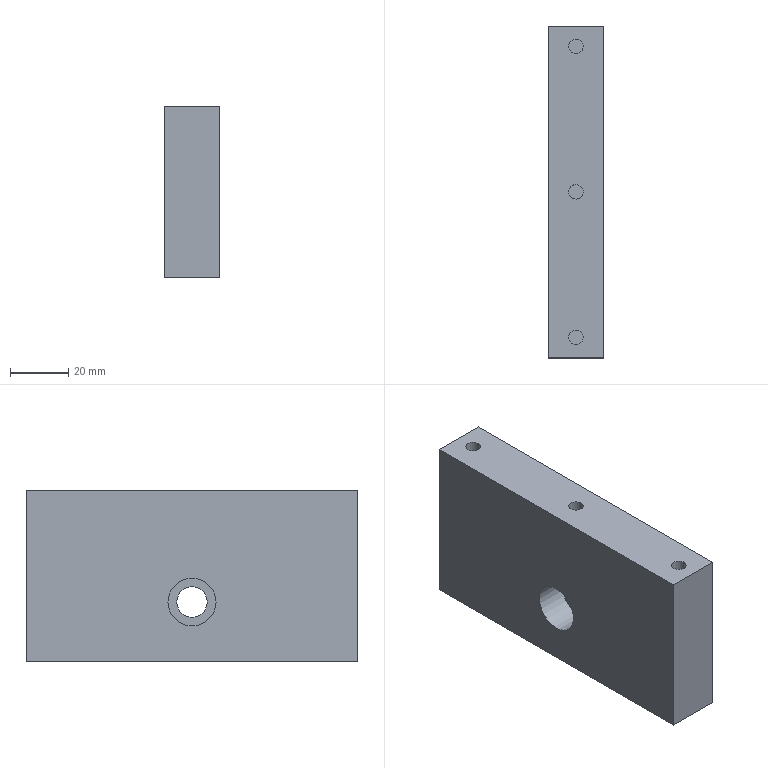Part | NX | 1 solid | 38 faces | box 19 x 114 x 59 mm | volume 122358 mm3 | plane 22 | cylinder 12 | cone 4 | commonest cylinder face diameters 5 x6 10.2 x4 10.5 x1 16.5 x1
STEP:
#1=CARTESIAN_POINT('',(808.094,637.643,-204.3));
#2=VERTEX_POINT('',#1);
#3=CARTESIAN_POINT('',(807.894,637.843,-204.3));
#4=VERTEX_POINT('',#3);
#5=CARTESIAN_POINT('',(808.094,637.643,-204.3));
#6=DIRECTION('',(-0.7071,0.7071,0.));
#7=VECTOR('',#6,1000.);
#8=LINE('',#5,#7);
#9=EDGE_CURVE('',#2,#4,#8,.T.);
#10=ORIENTED_EDGE('',*,*,#9,.T.);
#11=CARTESIAN_POINT('',(807.894,642.943,-199.2));
#12=VERTEX_POINT('',#11);
#13=CARTESIAN_POINT('',(807.894,642.943,-204.3));
#14=DIRECTION('',(1.,0.,0.));
#15=DIRECTION('',(0.,0.,1.));
#16=AXIS2_PLACEMENT_3D('',#13,#14,#15);
#17=CIRCLE('',#16,5.1);
#18=EDGE_CURVE('',#12,#4,#17,.T.);
#19=ORIENTED_EDGE('',*,*,#18,.F.);
#20=CARTESIAN_POINT('',(808.094,642.943,-199.));
#21=VERTEX_POINT('',#20);
#22=CARTESIAN_POINT('',(807.894,642.943,-199.2));
#23=DIRECTION('',(0.7071,0.,0.7071));
#24=VECTOR('',#23,1000.);
#25=LINE('',#22,#24);
#26=EDGE_CURVE('',#12,#21,#25,.T.);
#27=ORIENTED_EDGE('',*,*,#26,.T.);
#28=CARTESIAN_POINT('',(808.094,642.943,-204.3));
#29=DIRECTION('',(-1.,0.,0.));
#30=DIRECTION('',(0.,0.,1.));
#31=AXIS2_PLACEMENT_3D('',#28,#29,#30);
#32=CIRCLE('',#31,5.3);
#33=EDGE_CURVE('',#2,#21,#32,.T.);
#34=ORIENTED_EDGE('',*,*,#33,.F.);
#35=EDGE_LOOP('',(#10,#19,#27,#34));
#36=FACE_BOUND('',#35,.T.);
#37=CARTESIAN_POINT('',(808.094,642.943,-204.3));
#38=DIRECTION('',(1.,0.,0.));
#39=DIRECTION('',(0.,0.,-1.));
#40=AXIS2_PLACEMENT_3D('',#37,#38,#39);
#41=CONICAL_SURFACE('',#40,5.3,0.7854);
#42=ADVANCED_FACE('',(#36),#41,.F.);
#43=CARTESIAN_POINT('',(807.894,659.943,-199.2));
#44=VERTEX_POINT('',#43);
#45=CARTESIAN_POINT('',(808.094,659.943,-199.));
#46=VERTEX_POINT('',#45);
#47=CARTESIAN_POINT('',(807.894,659.943,-199.2));
#48=DIRECTION('',(0.7071,0.,0.7071));
#49=VECTOR('',#48,1000.);
#50=LINE('',#47,#49);
#51=EDGE_CURVE('',#44,#46,#50,.T.);
#52=ORIENTED_EDGE('',*,*,#51,.T.);
#53=CARTESIAN_POINT('',(808.094,606.293,-199.));
#54=DIRECTION('',(0.,1.,0.));
#55=VECTOR('',#54,1000.);
#56=LINE('',#53,#55);
#57=EDGE_CURVE('',#21,#46,#56,.T.);
#58=ORIENTED_EDGE('',*,*,#57,.F.);
#59=ORIENTED_EDGE('',*,*,#26,.F.);
#60=CARTESIAN_POINT('',(807.894,642.943,-199.2));
#61=DIRECTION('',(0.,-1.,0.));
#62=VECTOR('',#61,1000.);
#63=LINE('',#60,#62);
#64=EDGE_CURVE('',#44,#12,#63,.T.);
#65=ORIENTED_EDGE('',*,*,#64,.F.);
#66=EDGE_LOOP('',(#52,#58,#59,#65));
#67=FACE_BOUND('',#66,.T.);
#68=CARTESIAN_POINT('',(808.094,606.293,-199.));
#69=DIRECTION('',(-0.7071,0.,0.7071));
#70=DIRECTION('',(0.,1.,0.));
#71=AXIS2_PLACEMENT_3D('',#68,#69,#70);
#72=PLANE('',#71);
#73=ADVANCED_FACE('',(#67),#72,.F.);
#74=CARTESIAN_POINT('',(808.094,637.643,-211.3));
#75=VERTEX_POINT('',#74);
#76=CARTESIAN_POINT('',(807.894,637.843,-211.3));
#77=VERTEX_POINT('',#76);
#78=CARTESIAN_POINT('',(808.094,637.643,-211.3));
#79=DIRECTION('',(-0.7071,0.7071,0.));
#80=VECTOR('',#79,1000.);
#81=LINE('',#78,#80);
#82=EDGE_CURVE('',#75,#77,#81,.T.);
#83=ORIENTED_EDGE('',*,*,#82,.T.);
#84=CARTESIAN_POINT('',(807.894,637.843,-207.8));
#85=DIRECTION('',(0.,0.,-1.));
#86=VECTOR('',#85,1000.);
#87=LINE('',#84,#86);
#88=EDGE_CURVE('',#4,#77,#87,.T.);
#89=ORIENTED_EDGE('',*,*,#88,.F.);
#90=ORIENTED_EDGE('',*,*,#9,.F.);
#91=CARTESIAN_POINT('',(808.094,637.643,-230.3));
#92=DIRECTION('',(0.,0.,1.));
#93=VECTOR('',#92,1000.);
#94=LINE('',#91,#93);
#95=EDGE_CURVE('',#75,#2,#94,.T.);
#96=ORIENTED_EDGE('',*,*,#95,.F.);
#97=EDGE_LOOP('',(#83,#89,#90,#96));
#98=FACE_BOUND('',#97,.T.);
#99=CARTESIAN_POINT('',(808.094,637.643,-230.3));
#100=DIRECTION('',(-0.7071,-0.7071,0.));
#101=DIRECTION('',(0.,0.,1.));
#102=AXIS2_PLACEMENT_3D('',#99,#100,#101);
#103=PLANE('',#102);
#104=ADVANCED_FACE('',(#98),#103,.F.);
#105=CARTESIAN_POINT('',(807.894,665.043,-204.3));
#106=VERTEX_POINT('',#105);
#107=CARTESIAN_POINT('',(808.094,665.243,-204.3));
#108=VERTEX_POINT('',#107);
#109=CARTESIAN_POINT('',(807.894,665.043,-204.3));
#110=DIRECTION('',(0.7071,0.7071,0.));
#111=VECTOR('',#110,1000.);
#112=LINE('',#109,#111);
#113=EDGE_CURVE('',#106,#108,#112,.T.);
#114=ORIENTED_EDGE('',*,*,#113,.T.);
#115=CARTESIAN_POINT('',(808.094,659.943,-204.3));
#116=DIRECTION('',(-1.,0.,0.));
#117=DIRECTION('',(0.,0.,1.));
#118=AXIS2_PLACEMENT_3D('',#115,#116,#117);
#119=CIRCLE('',#118,5.3);
#120=EDGE_CURVE('',#46,#108,#119,.T.);
#121=ORIENTED_EDGE('',*,*,#120,.F.);
#122=ORIENTED_EDGE('',*,*,#51,.F.);
#123=CARTESIAN_POINT('',(807.894,659.943,-204.3));
#124=DIRECTION('',(1.,0.,0.));
#125=DIRECTION('',(0.,0.,1.));
#126=AXIS2_PLACEMENT_3D('',#123,#124,#125);
#127=CIRCLE('',#126,5.1);
#128=EDGE_CURVE('',#106,#44,#127,.T.);
#129=ORIENTED_EDGE('',*,*,#128,.F.);
#130=EDGE_LOOP('',(#114,#121,#122,#129));
#131=FACE_BOUND('',#130,.T.);
#132=CARTESIAN_POINT('',(808.094,659.943,-204.3));
#133=DIRECTION('',(1.,0.,0.));
#134=DIRECTION('',(0.,0.,-1.));
#135=AXIS2_PLACEMENT_3D('',#132,#133,#134);
#136=CONICAL_SURFACE('',#135,5.3,0.7854);
#137=ADVANCED_FACE('',(#131),#136,.F.);
#138=CARTESIAN_POINT('',(808.094,642.943,-216.6));
#139=VERTEX_POINT('',#138);
#140=CARTESIAN_POINT('',(807.894,642.943,-216.4));
#141=VERTEX_POINT('',#140);
#142=CARTESIAN_POINT('',(808.094,642.943,-216.6));
#143=DIRECTION('',(-0.7071,0.,0.7071));
#144=VECTOR('',#143,1000.);
#145=LINE('',#142,#144);
#146=EDGE_CURVE('',#139,#141,#145,.T.);
#147=ORIENTED_EDGE('',*,*,#146,.T.);
#148=CARTESIAN_POINT('',(807.894,642.943,-211.3));
#149=DIRECTION('',(1.,0.,0.));
#150=DIRECTION('',(0.,0.,1.));
#151=AXIS2_PLACEMENT_3D('',#148,#149,#150);
#152=CIRCLE('',#151,5.1);
#153=EDGE_CURVE('',#77,#141,#152,.T.);
#154=ORIENTED_EDGE('',*,*,#153,.F.);
#155=ORIENTED_EDGE('',*,*,#82,.F.);
#156=CARTESIAN_POINT('',(808.094,642.943,-211.3));
#157=DIRECTION('',(-1.,0.,0.));
#158=DIRECTION('',(0.,0.,1.));
#159=AXIS2_PLACEMENT_3D('',#156,#157,#158);
#160=CIRCLE('',#159,5.3);
#161=EDGE_CURVE('',#139,#75,#160,.T.);
#162=ORIENTED_EDGE('',*,*,#161,.F.);
#163=EDGE_LOOP('',(#147,#154,#155,#162));
#164=FACE_BOUND('',#163,.T.);
#165=CARTESIAN_POINT('',(808.094,642.943,-211.3));
#166=DIRECTION('',(1.,0.,0.));
#167=DIRECTION('',(0.,0.,-1.));
#168=AXIS2_PLACEMENT_3D('',#165,#166,#167);
#169=CONICAL_SURFACE('',#168,5.3,0.7854);
#170=ADVANCED_FACE('',(#164),#169,.F.);
#171=CARTESIAN_POINT('',(807.894,665.043,-211.3));
#172=VERTEX_POINT('',#171);
#173=CARTESIAN_POINT('',(808.094,665.243,-211.3));
#174=VERTEX_POINT('',#173);
#175=CARTESIAN_POINT('',(807.894,665.043,-211.3));
#176=DIRECTION('',(0.7071,0.7071,0.));
#177=VECTOR('',#176,1000.);
#178=LINE('',#175,#177);
#179=EDGE_CURVE('',#172,#174,#178,.T.);
#180=ORIENTED_EDGE('',*,*,#179,.T.);
#181=CARTESIAN_POINT('',(808.094,665.243,-230.3));
#182=DIRECTION('',(0.,0.,-1.));
#183=VECTOR('',#182,1000.);
#184=LINE('',#181,#183);
#185=EDGE_CURVE('',#108,#174,#184,.T.);
#186=ORIENTED_EDGE('',*,*,#185,.F.);
#187=ORIENTED_EDGE('',*,*,#113,.F.);
#188=CARTESIAN_POINT('',(807.894,665.043,-207.8));
#189=DIRECTION('',(0.,0.,1.));
#190=VECTOR('',#189,1000.);
#191=LINE('',#188,#190);
#192=EDGE_CURVE('',#172,#106,#191,.T.);
#193=ORIENTED_EDGE('',*,*,#192,.F.);
#194=EDGE_LOOP('',(#180,#186,#187,#193));
#195=FACE_BOUND('',#194,.T.);
#196=CARTESIAN_POINT('',(808.094,665.243,-230.3));
#197=DIRECTION('',(-0.7071,0.7071,0.));
#198=DIRECTION('',(0.,0.,-1.));
#199=AXIS2_PLACEMENT_3D('',#196,#197,#198);
#200=PLANE('',#199);
#201=ADVANCED_FACE('',(#195),#200,.F.);
#202=CARTESIAN_POINT('',(808.094,659.943,-216.6));
#203=VERTEX_POINT('',#202);
#204=CARTESIAN_POINT('',(807.894,659.943,-216.4));
#205=VERTEX_POINT('',#204);
#206=CARTESIAN_POINT('',(808.094,659.943,-216.6));
#207=DIRECTION('',(-0.7071,0.,0.7071));
#208=VECTOR('',#207,1000.);
#209=LINE('',#206,#208);
#210=EDGE_CURVE('',#203,#205,#209,.T.);
#211=ORIENTED_EDGE('',*,*,#210,.T.);
#212=CARTESIAN_POINT('',(807.894,642.943,-216.4));
#213=DIRECTION('',(0.,1.,0.));
#214=VECTOR('',#213,1000.);
#215=LINE('',#212,#214);
#216=EDGE_CURVE('',#141,#205,#215,.T.);
#217=ORIENTED_EDGE('',*,*,#216,.F.);
#218=ORIENTED_EDGE('',*,*,#146,.F.);
#219=CARTESIAN_POINT('',(808.094,606.293,-216.6));
#220=DIRECTION('',(0.,-1.,0.));
#221=VECTOR('',#220,1000.);
#222=LINE('',#219,#221);
#223=EDGE_CURVE('',#203,#139,#222,.T.);
#224=ORIENTED_EDGE('',*,*,#223,.F.);
#225=EDGE_LOOP('',(#211,#217,#218,#224));
#226=FACE_BOUND('',#225,.T.);
#227=CARTESIAN_POINT('',(808.094,606.293,-216.6));
#228=DIRECTION('',(-0.7071,0.,-0.7071));
#229=DIRECTION('',(0.,-1.,0.));
#230=AXIS2_PLACEMENT_3D('',#227,#228,#229);
#231=PLANE('',#230);
#232=ADVANCED_FACE('',(#226),#231,.F.);
#233=ORIENTED_EDGE('',*,*,#179,.F.);
#234=CARTESIAN_POINT('',(807.894,659.943,-211.3));
#235=DIRECTION('',(1.,0.,0.));
#236=DIRECTION('',(0.,0.,1.));
#237=AXIS2_PLACEMENT_3D('',#234,#235,#236);
#238=CIRCLE('',#237,5.1);
#239=EDGE_CURVE('',#205,#172,#238,.T.);
#240=ORIENTED_EDGE('',*,*,#239,.F.);
#241=ORIENTED_EDGE('',*,*,#210,.F.);
#242=CARTESIAN_POINT('',(808.094,659.943,-211.3));
#243=DIRECTION('',(-1.,0.,0.));
#244=DIRECTION('',(0.,0.,1.));
#245=AXIS2_PLACEMENT_3D('',#242,#243,#244);
#246=CIRCLE('',#245,5.3);
#247=EDGE_CURVE('',#174,#203,#246,.T.);
#248=ORIENTED_EDGE('',*,*,#247,.F.);
#249=EDGE_LOOP('',(#233,#240,#241,#248));
#250=FACE_BOUND('',#249,.T.);
#251=CARTESIAN_POINT('',(808.094,659.943,-211.3));
#252=DIRECTION('',(1.,0.,0.));
#253=DIRECTION('',(0.,0.,-1.));
#254=AXIS2_PLACEMENT_3D('',#251,#252,#253);
#255=CONICAL_SURFACE('',#254,5.3,0.7854);
#256=ADVANCED_FACE('',(#250),#255,.F.);
#257=CARTESIAN_POINT('',(796.094,701.443,-184.35));
#258=VERTEX_POINT('',#257);
#259=CARTESIAN_POINT('',(798.594,701.443,-184.35));
#260=DIRECTION('',(0.,0.,-1.));
#261=DIRECTION('',(-1.,0.,0.));
#262=AXIS2_PLACEMENT_3D('',#259,#260,#261);
#263=CIRCLE('',#262,2.5);
#264=EDGE_CURVE('',#258,#258,#263,.T.);
#265=ORIENTED_EDGE('',*,*,#264,.F.);
#266=EDGE_LOOP('',(#265));
#267=FACE_BOUND('',#266,.T.);
#268=CARTESIAN_POINT('',(798.594,638.943,-184.35));
#269=DIRECTION('',(0.,0.,-1.));
#270=DIRECTION('',(0.,-1.,0.));
#271=AXIS2_PLACEMENT_3D('',#268,#269,#270);
#272=PLANE('',#271);
#273=ADVANCED_FACE('',(#267),#272,.F.);
#274=ORIENTED_EDGE('',*,*,#264,.T.);
#275=EDGE_LOOP('',(#274));
#276=FACE_BOUND('',#275,.T.);
#277=CARTESIAN_POINT('',(798.594,698.943,-169.35));
#278=VERTEX_POINT('',#277);
#279=CARTESIAN_POINT('',(798.594,701.443,-169.35));
#280=DIRECTION('',(0.,0.,1.));
#281=DIRECTION('',(0.,-1.,0.));
#282=AXIS2_PLACEMENT_3D('',#279,#280,#281);
#283=CIRCLE('',#282,2.5);
#284=EDGE_CURVE('',#278,#278,#283,.T.);
#285=ORIENTED_EDGE('',*,*,#284,.T.);
#286=EDGE_LOOP('',(#285));
#287=FACE_BOUND('',#286,.T.);
#288=CARTESIAN_POINT('',(798.594,701.443,-184.35));
#289=DIRECTION('',(0.,0.,1.));
#290=DIRECTION('',(-1.,0.,0.));
#291=AXIS2_PLACEMENT_3D('',#288,#289,#290);
#292=CYLINDRICAL_SURFACE('',#291,2.5);
#293=ADVANCED_FACE('',(#276,#287),#292,.F.);
#294=CARTESIAN_POINT('',(796.094,601.443,-184.35));
#295=VERTEX_POINT('',#294);
#296=CARTESIAN_POINT('',(798.594,601.443,-184.35));
#297=DIRECTION('',(0.,0.,-1.));
#298=DIRECTION('',(-1.,0.,0.));
#299=AXIS2_PLACEMENT_3D('',#296,#297,#298);
#300=CIRCLE('',#299,2.5);
#301=EDGE_CURVE('',#295,#295,#300,.T.);
#302=ORIENTED_EDGE('',*,*,#301,.F.);
#303=EDGE_LOOP('',(#302));
#304=FACE_BOUND('',#303,.T.);
#305=CARTESIAN_POINT('',(798.594,638.943,-184.35));
#306=DIRECTION('',(0.,0.,-1.));
#307=DIRECTION('',(0.,-1.,0.));
#308=AXIS2_PLACEMENT_3D('',#305,#306,#307);
#309=PLANE('',#308);
#310=ADVANCED_FACE('',(#304),#309,.F.);
#311=ORIENTED_EDGE('',*,*,#301,.T.);
#312=EDGE_LOOP('',(#311));
#313=FACE_BOUND('',#312,.T.);
#314=CARTESIAN_POINT('',(798.594,598.943,-169.35));
#315=VERTEX_POINT('',#314);
#316=CARTESIAN_POINT('',(798.594,601.443,-169.35));
#317=DIRECTION('',(0.,0.,1.));
#318=DIRECTION('',(0.,-1.,0.));
#319=AXIS2_PLACEMENT_3D('',#316,#317,#318);
#320=CIRCLE('',#319,2.5);
#321=EDGE_CURVE('',#315,#315,#320,.T.);
#322=ORIENTED_EDGE('',*,*,#321,.T.);
#323=EDGE_LOOP('',(#322));
#324=FACE_BOUND('',#323,.T.);
#325=CARTESIAN_POINT('',(798.594,601.443,-184.35));
#326=DIRECTION('',(0.,0.,1.));
#327=DIRECTION('',(-1.,0.,0.));
#328=AXIS2_PLACEMENT_3D('',#325,#326,#327);
#329=CYLINDRICAL_SURFACE('',#328,2.5);
#330=ADVANCED_FACE('',(#313,#324),#329,.F.);
#331=CARTESIAN_POINT('',(796.094,651.443,-184.35));
#332=VERTEX_POINT('',#331);
#333=CARTESIAN_POINT('',(798.594,651.443,-184.35));
#334=DIRECTION('',(0.,0.,-1.));
#335=DIRECTION('',(-1.,0.,0.));
#336=AXIS2_PLACEMENT_3D('',#333,#334,#335);
#337=CIRCLE('',#336,2.5);
#338=EDGE_CURVE('',#332,#332,#337,.T.);
#339=ORIENTED_EDGE('',*,*,#338,.T.);
#340=EDGE_LOOP('',(#339));
#341=FACE_BOUND('',#340,.T.);
#342=CARTESIAN_POINT('',(798.594,648.943,-169.35));
#343=VERTEX_POINT('',#342);
#344=CARTESIAN_POINT('',(798.594,651.443,-169.35));
#345=DIRECTION('',(0.,0.,-1.));
#346=DIRECTION('',(0.,-1.,0.));
#347=AXIS2_PLACEMENT_3D('',#344,#345,#346);
#348=CIRCLE('',#347,2.5);
#349=EDGE_CURVE('',#343,#343,#348,.T.);
#350=ORIENTED_EDGE('',*,*,#349,.F.);
#351=EDGE_LOOP('',(#350));
#352=FACE_BOUND('',#351,.T.);
#353=CARTESIAN_POINT('',(798.594,651.443,-184.35));
#354=DIRECTION('',(0.,0.,1.));
#355=DIRECTION('',(-1.,0.,0.));
#356=AXIS2_PLACEMENT_3D('',#353,#354,#355);
#357=CYLINDRICAL_SURFACE('',#356,2.5);
#358=ADVANCED_FACE('',(#341,#352),#357,.F.);
#359=ORIENTED_EDGE('',*,*,#338,.F.);
#360=EDGE_LOOP('',(#359));
#361=FACE_BOUND('',#360,.T.);
#362=CARTESIAN_POINT('',(798.594,638.943,-184.35));
#363=DIRECTION('',(0.,0.,-1.));
#364=DIRECTION('',(0.,-1.,0.));
#365=AXIS2_PLACEMENT_3D('',#362,#363,#364);
#366=PLANE('',#365);
#367=ADVANCED_FACE('',(#361),#366,.F.);
#368=CARTESIAN_POINT('',(801.094,601.443,-228.35));
#369=VERTEX_POINT('',#368);
#370=CARTESIAN_POINT('',(798.594,601.443,-228.35));
#371=DIRECTION('',(0.,0.,1.));
#372=DIRECTION('',(1.,0.,0.));
#373=AXIS2_PLACEMENT_3D('',#370,#371,#372);
#374=CIRCLE('',#373,2.5);
#375=EDGE_CURVE('',#369,#369,#374,.T.);
#376=ORIENTED_EDGE('',*,*,#375,.F.);
#377=EDGE_LOOP('',(#376));
#378=FACE_BOUND('',#377,.T.);
#379=CARTESIAN_POINT('',(801.094,601.443,-213.3));
#380=VERTEX_POINT('',#379);
#381=CARTESIAN_POINT('',(798.594,601.443,-213.3));
#382=DIRECTION('',(0.,0.,1.));
#383=DIRECTION('',(1.,0.,0.));
#384=AXIS2_PLACEMENT_3D('',#381,#382,#383);
#385=CIRCLE('',#384,2.5);
#386=EDGE_CURVE('',#380,#380,#385,.T.);
#387=ORIENTED_EDGE('',*,*,#386,.T.);
#388=EDGE_LOOP('',(#387));
#389=FACE_BOUND('',#388,.T.);
#390=CARTESIAN_POINT('',(798.594,601.443,-184.35));
#391=DIRECTION('',(0.,0.,1.));
#392=DIRECTION('',(-1.,0.,0.));
#393=AXIS2_PLACEMENT_3D('',#390,#391,#392);
#394=CYLINDRICAL_SURFACE('',#393,2.5);
#395=ADVANCED_FACE('',(#378,#389),#394,.F.);
#396=ORIENTED_EDGE('',*,*,#386,.F.);
#397=EDGE_LOOP('',(#396));
#398=FACE_BOUND('',#397,.T.);
#399=CARTESIAN_POINT('',(798.594,601.443,-213.3));
#400=DIRECTION('',(0.,0.,1.));
#401=DIRECTION('',(0.,1.,0.));
#402=AXIS2_PLACEMENT_3D('',#399,#400,#401);
#403=PLANE('',#402);
#404=ADVANCED_FACE('',(#398),#403,.F.);
#405=CARTESIAN_POINT('',(801.094,701.443,-228.35));
#406=VERTEX_POINT('',#405);
#407=CARTESIAN_POINT('',(798.594,701.443,-228.35));
#408=DIRECTION('',(0.,0.,1.));
#409=DIRECTION('',(1.,0.,0.));
#410=AXIS2_PLACEMENT_3D('',#407,#408,#409);
#411=CIRCLE('',#410,2.5);
#412=EDGE_CURVE('',#406,#406,#411,.T.);
#413=ORIENTED_EDGE('',*,*,#412,.F.);
#414=EDGE_LOOP('',(#413));
#415=FACE_BOUND('',#414,.T.);
#416=CARTESIAN_POINT('',(801.094,701.443,-213.3));
#417=VERTEX_POINT('',#416);
#418=CARTESIAN_POINT('',(798.594,701.443,-213.3));
#419=DIRECTION('',(0.,0.,1.));
#420=DIRECTION('',(1.,0.,0.));
#421=AXIS2_PLACEMENT_3D('',#418,#419,#420);
#422=CIRCLE('',#421,2.5);
#423=EDGE_CURVE('',#417,#417,#422,.T.);
#424=ORIENTED_EDGE('',*,*,#423,.T.);
#425=EDGE_LOOP('',(#424));
#426=FACE_BOUND('',#425,.T.);
#427=CARTESIAN_POINT('',(798.594,701.443,-184.35));
#428=DIRECTION('',(0.,0.,1.));
#429=DIRECTION('',(-1.,0.,0.));
#430=AXIS2_PLACEMENT_3D('',#427,#428,#429);
#431=CYLINDRICAL_SURFACE('',#430,2.5);
#432=ADVANCED_FACE('',(#415,#426),#431,.F.);
#433=ORIENTED_EDGE('',*,*,#423,.F.);
#434=EDGE_LOOP('',(#433));
#435=FACE_BOUND('',#434,.T.);
#436=CARTESIAN_POINT('',(798.594,601.443,-213.3));
#437=DIRECTION('',(0.,0.,1.));
#438=DIRECTION('',(0.,1.,0.));
#439=AXIS2_PLACEMENT_3D('',#436,#437,#438);
#440=PLANE('',#439);
#441=ADVANCED_FACE('',(#435),#440,.F.);
#442=CARTESIAN_POINT('',(801.094,651.443,-228.35));
#443=VERTEX_POINT('',#442);
#444=CARTESIAN_POINT('',(798.594,651.443,-228.35));
#445=DIRECTION('',(0.,0.,1.));
#446=DIRECTION('',(1.,0.,0.));
#447=AXIS2_PLACEMENT_3D('',#444,#445,#446);
#448=CIRCLE('',#447,2.5);
#449=EDGE_CURVE('',#443,#443,#448,.T.);
#450=ORIENTED_EDGE('',*,*,#449,.F.);
#451=EDGE_LOOP('',(#450));
#452=FACE_BOUND('',#451,.T.);
#453=CARTESIAN_POINT('',(801.094,651.443,-218.3));
#454=VERTEX_POINT('',#453);
#455=CARTESIAN_POINT('',(798.594,651.443,-218.3));
#456=DIRECTION('',(0.,0.,1.));
#457=DIRECTION('',(1.,0.,0.));
#458=AXIS2_PLACEMENT_3D('',#455,#456,#457);
#459=CIRCLE('',#458,2.5);
#460=EDGE_CURVE('',#454,#454,#459,.T.);
#461=ORIENTED_EDGE('',*,*,#460,.T.);
#462=EDGE_LOOP('',(#461));
#463=FACE_BOUND('',#462,.T.);
#464=CARTESIAN_POINT('',(798.594,651.443,-184.35));
#465=DIRECTION('',(0.,0.,1.));
#466=DIRECTION('',(-1.,0.,0.));
#467=AXIS2_PLACEMENT_3D('',#464,#465,#466);
#468=CYLINDRICAL_SURFACE('',#467,2.5);
#469=ADVANCED_FACE('',(#452,#463),#468,.F.);
#470=ORIENTED_EDGE('',*,*,#460,.F.);
#471=EDGE_LOOP('',(#470));
#472=FACE_BOUND('',#471,.T.);
#473=CARTESIAN_POINT('',(798.594,651.443,-218.3));
#474=DIRECTION('',(0.,0.,1.));
#475=DIRECTION('',(0.,1.,0.));
#476=AXIS2_PLACEMENT_3D('',#473,#474,#475);
#477=PLANE('',#476);
#478=ADVANCED_FACE('',(#472),#477,.F.);
#479=CARTESIAN_POINT('',(800.094,646.193,-207.8));
#480=VERTEX_POINT('',#479);
#481=CARTESIAN_POINT('',(800.094,651.443,-207.8));
#482=DIRECTION('',(1.,0.,0.));
#483=DIRECTION('',(0.,-1.,0.));
#484=AXIS2_PLACEMENT_3D('',#481,#482,#483);
#485=CIRCLE('',#484,5.25);
#486=EDGE_CURVE('',#480,#480,#485,.T.);
#487=ORIENTED_EDGE('',*,*,#486,.T.);
#488=EDGE_LOOP('',(#487));
#489=FACE_BOUND('',#488,.T.);
#490=CARTESIAN_POINT('',(800.094,643.193,-207.8));
#491=VERTEX_POINT('',#490);
#492=CARTESIAN_POINT('',(800.094,651.443,-207.8));
#493=DIRECTION('',(-1.,0.,0.));
#494=DIRECTION('',(0.,-1.,0.));
#495=AXIS2_PLACEMENT_3D('',#492,#493,#494);
#496=CIRCLE('',#495,8.25);
#497=EDGE_CURVE('',#491,#491,#496,.T.);
#498=ORIENTED_EDGE('',*,*,#497,.T.);
#499=EDGE_LOOP('',(#498));
#500=FACE_BOUND('',#499,.T.);
#501=CARTESIAN_POINT('',(800.094,651.443,-198.825));
#502=DIRECTION('',(-1.,0.,0.));
#503=DIRECTION('',(0.,-1.,0.));
#504=AXIS2_PLACEMENT_3D('',#501,#502,#503);
#505=PLANE('',#504);
#506=ADVANCED_FACE('',(#489,#500),#505,.T.);
#507=CARTESIAN_POINT('',(806.094,642.943,-199.2));
#508=VERTEX_POINT('',#507);
#509=CARTESIAN_POINT('',(810.094,642.943,-199.2));
#510=DIRECTION('',(-1.,0.,0.));
#511=VECTOR('',#510,1000.);
#512=LINE('',#509,#511);
#513=EDGE_CURVE('',#12,#508,#512,.T.);
#514=ORIENTED_EDGE('',*,*,#513,.F.);
#515=ORIENTED_EDGE('',*,*,#18,.T.);
#516=CARTESIAN_POINT('',(806.094,637.843,-204.3));
#517=VERTEX_POINT('',#516);
#518=CARTESIAN_POINT('',(810.094,637.843,-204.3));
#519=DIRECTION('',(1.,0.,0.));
#520=VECTOR('',#519,1000.);
#521=LINE('',#518,#520);
#522=EDGE_CURVE('',#517,#4,#521,.T.);
#523=ORIENTED_EDGE('',*,*,#522,.F.);
#524=CARTESIAN_POINT('',(806.094,642.943,-204.3));
#525=DIRECTION('',(1.,0.,0.));
#526=DIRECTION('',(0.,0.,1.));
#527=AXIS2_PLACEMENT_3D('',#524,#525,#526);
#528=CIRCLE('',#527,5.1);
#529=EDGE_CURVE('',#508,#517,#528,.T.);
#530=ORIENTED_EDGE('',*,*,#529,.F.);
#531=EDGE_LOOP('',(#514,#515,#523,#530));
#532=FACE_BOUND('',#531,.T.);
#533=CARTESIAN_POINT('',(810.094,642.943,-204.3));
#534=DIRECTION('',(1.,0.,0.));
#535=DIRECTION('',(0.,1.,0.));
#536=AXIS2_PLACEMENT_3D('',#533,#534,#535);
#537=CYLINDRICAL_SURFACE('',#536,5.1);
#538=ADVANCED_FACE('',(#532),#537,.F.);
#539=CARTESIAN_POINT('',(806.094,637.843,-211.3));
#540=VERTEX_POINT('',#539);
#541=CARTESIAN_POINT('',(810.094,637.843,-211.3));
#542=DIRECTION('',(-1.,0.,0.));
#543=VECTOR('',#542,1000.);
#544=LINE('',#541,#543);
#545=EDGE_CURVE('',#77,#540,#544,.T.);
#546=ORIENTED_EDGE('',*,*,#545,.F.);
#547=ORIENTED_EDGE('',*,*,#153,.T.);
#548=CARTESIAN_POINT('',(806.094,642.943,-216.4));
#549=VERTEX_POINT('',#548);
#550=CARTESIAN_POINT('',(810.094,642.943,-216.4));
#551=DIRECTION('',(1.,0.,0.));
#552=VECTOR('',#551,1000.);
#553=LINE('',#550,#552);
#554=EDGE_CURVE('',#549,#141,#553,.T.);
#555=ORIENTED_EDGE('',*,*,#554,.F.);
#556=CARTESIAN_POINT('',(806.094,642.943,-211.3));
#557=DIRECTION('',(1.,0.,0.));
#558=DIRECTION('',(0.,0.,1.));
#559=AXIS2_PLACEMENT_3D('',#556,#557,#558);
#560=CIRCLE('',#559,5.1);
#561=EDGE_CURVE('',#540,#549,#560,.T.);
#562=ORIENTED_EDGE('',*,*,#561,.F.);
#563=EDGE_LOOP('',(#546,#547,#555,#562));
#564=FACE_BOUND('',#563,.T.);
#565=CARTESIAN_POINT('',(810.094,642.943,-211.3));
#566=DIRECTION('',(-1.,0.,0.));
#567=DIRECTION('',(0.,-1.,0.));
#568=AXIS2_PLACEMENT_3D('',#565,#566,#567);
#569=CYLINDRICAL_SURFACE('',#568,5.1);
#570=ADVANCED_FACE('',(#564),#569,.F.);
#571=CARTESIAN_POINT('',(806.094,665.043,-204.3));
#572=VERTEX_POINT('',#571);
#573=CARTESIAN_POINT('',(810.094,665.043,-204.3));
#574=DIRECTION('',(-1.,0.,0.));
#575=VECTOR('',#574,1000.);
#576=LINE('',#573,#575);
#577=EDGE_CURVE('',#106,#572,#576,.T.);
#578=ORIENTED_EDGE('',*,*,#577,.F.);
#579=ORIENTED_EDGE('',*,*,#128,.T.);
#580=CARTESIAN_POINT('',(806.094,659.943,-199.2));
#581=VERTEX_POINT('',#580);
#582=CARTESIAN_POINT('',(810.094,659.943,-199.2));
#583=DIRECTION('',(1.,0.,0.));
#584=VECTOR('',#583,1000.);
#585=LINE('',#582,#584);
#586=EDGE_CURVE('',#581,#44,#585,.T.);
#587=ORIENTED_EDGE('',*,*,#586,.F.);
#588=CARTESIAN_POINT('',(806.094,659.943,-204.3));
#589=DIRECTION('',(1.,0.,0.));
#590=DIRECTION('',(0.,0.,1.));
#591=AXIS2_PLACEMENT_3D('',#588,#589,#590);
#592=CIRCLE('',#591,5.1);
#593=EDGE_CURVE('',#572,#581,#592,.T.);
#594=ORIENTED_EDGE('',*,*,#593,.F.);
#595=EDGE_LOOP('',(#578,#579,#587,#594));
#596=FACE_BOUND('',#595,.T.);
#597=CARTESIAN_POINT('',(810.094,659.943,-204.3));
#598=DIRECTION('',(-1.,0.,0.));
#599=DIRECTION('',(0.,-1.,0.));
#600=AXIS2_PLACEMENT_3D('',#597,#598,#599);
#601=CYLINDRICAL_SURFACE('',#600,5.1);
#602=ADVANCED_FACE('',(#596),#601,.F.);
#603=CARTESIAN_POINT('',(806.094,659.943,-216.4));
#604=VERTEX_POINT('',#603);
#605=CARTESIAN_POINT('',(810.094,659.943,-216.4));
#606=DIRECTION('',(-1.,0.,0.));
#607=VECTOR('',#606,1000.);
#608=LINE('',#605,#607);
#609=EDGE_CURVE('',#205,#604,#608,.T.);
#610=ORIENTED_EDGE('',*,*,#609,.F.);
#611=ORIENTED_EDGE('',*,*,#239,.T.);
#612=CARTESIAN_POINT('',(806.094,665.043,-211.3));
#613=VERTEX_POINT('',#612);
#614=CARTESIAN_POINT('',(810.094,665.043,-211.3));
#615=DIRECTION('',(1.,0.,0.));
#616=VECTOR('',#615,1000.);
#617=LINE('',#614,#616);
#618=EDGE_CURVE('',#613,#172,#617,.T.);
#619=ORIENTED_EDGE('',*,*,#618,.F.);
#620=CARTESIAN_POINT('',(806.094,659.943,-211.3));
#621=DIRECTION('',(1.,0.,0.));
#622=DIRECTION('',(0.,0.,1.));
#623=AXIS2_PLACEMENT_3D('',#620,#621,#622);
#624=CIRCLE('',#623,5.1);
#625=EDGE_CURVE('',#604,#613,#624,.T.);
#626=ORIENTED_EDGE('',*,*,#625,.F.);
#627=EDGE_LOOP('',(#610,#611,#619,#626));
#628=FACE_BOUND('',#627,.T.);
#629=CARTESIAN_POINT('',(810.094,659.943,-211.3));
#630=DIRECTION('',(1.,0.,0.));
#631=DIRECTION('',(0.,1.,0.));
#632=AXIS2_PLACEMENT_3D('',#629,#630,#631);
#633=CYLINDRICAL_SURFACE('',#632,5.1);
#634=ADVANCED_FACE('',(#628),#633,.F.);
#635=CARTESIAN_POINT('',(806.094,637.843,-207.8));
#636=DIRECTION('',(0.,0.,-1.));
#637=VECTOR('',#636,1000.);
#638=LINE('',#635,#637);
#639=EDGE_CURVE('',#517,#540,#638,.T.);
#640=ORIENTED_EDGE('',*,*,#639,.T.);
#641=ORIENTED_EDGE('',*,*,#561,.T.);
#642=CARTESIAN_POINT('',(806.094,642.943,-216.4));
#643=DIRECTION('',(0.,-1.,0.));
#644=VECTOR('',#643,1000.);
#645=LINE('',#642,#644);
#646=EDGE_CURVE('',#604,#549,#645,.T.);
#647=ORIENTED_EDGE('',*,*,#646,.F.);
#648=ORIENTED_EDGE('',*,*,#625,.T.);
#649=CARTESIAN_POINT('',(806.094,665.043,-207.8));
#650=DIRECTION('',(0.,0.,1.));
#651=VECTOR('',#650,1000.);
#652=LINE('',#649,#651);
#653=EDGE_CURVE('',#613,#572,#652,.T.);
#654=ORIENTED_EDGE('',*,*,#653,.T.);
#655=ORIENTED_EDGE('',*,*,#593,.T.);
#656=CARTESIAN_POINT('',(806.094,642.943,-199.2));
#657=DIRECTION('',(0.,-1.,0.));
#658=VECTOR('',#657,1000.);
#659=LINE('',#656,#658);
#660=EDGE_CURVE('',#581,#508,#659,.T.);
#661=ORIENTED_EDGE('',*,*,#660,.T.);
#662=ORIENTED_EDGE('',*,*,#529,.T.);
#663=EDGE_LOOP('',(#640,#641,#647,#648,#654,#655,#661,#662));
#664=FACE_BOUND('',#663,.T.);
#665=CARTESIAN_POINT('',(806.094,646.193,-207.8));
#666=VERTEX_POINT('',#665);
#667=CARTESIAN_POINT('',(806.094,651.443,-207.8));
#668=DIRECTION('',(1.,0.,0.));
#669=DIRECTION('',(0.,-1.,0.));
#670=AXIS2_PLACEMENT_3D('',#667,#668,#669);
#671=CIRCLE('',#670,5.25);
#672=EDGE_CURVE('',#666,#666,#671,.T.);
#673=ORIENTED_EDGE('',*,*,#672,.F.);
#674=EDGE_LOOP('',(#673));
#675=FACE_BOUND('',#674,.T.);
#676=CARTESIAN_POINT('',(806.094,642.943,-207.8));
#677=DIRECTION('',(-1.,0.,0.));
#678=DIRECTION('',(0.,-1.,0.));
#679=AXIS2_PLACEMENT_3D('',#676,#677,#678);
#680=PLANE('',#679);
#681=ADVANCED_FACE('',(#664,#675),#680,.F.);
#682=ORIENTED_EDGE('',*,*,#522,.T.);
#683=ORIENTED_EDGE('',*,*,#88,.T.);
#684=ORIENTED_EDGE('',*,*,#545,.T.);
#685=ORIENTED_EDGE('',*,*,#639,.F.);
#686=EDGE_LOOP('',(#682,#683,#684,#685));
#687=FACE_BOUND('',#686,.T.);
#688=CARTESIAN_POINT('',(810.094,637.843,-207.8));
#689=DIRECTION('',(0.,-1.,0.));
#690=DIRECTION('',(1.,0.,0.));
#691=AXIS2_PLACEMENT_3D('',#688,#689,#690);
#692=PLANE('',#691);
#693=ADVANCED_FACE('',(#687),#692,.F.);
#694=ORIENTED_EDGE('',*,*,#586,.T.);
#695=ORIENTED_EDGE('',*,*,#64,.T.);
#696=ORIENTED_EDGE('',*,*,#513,.T.);
#697=ORIENTED_EDGE('',*,*,#660,.F.);
#698=EDGE_LOOP('',(#694,#695,#696,#697));
#699=FACE_BOUND('',#698,.T.);
#700=CARTESIAN_POINT('',(810.094,642.943,-199.2));
#701=DIRECTION('',(0.,0.,1.));
#702=DIRECTION('',(0.,1.,0.));
#703=AXIS2_PLACEMENT_3D('',#700,#701,#702);
#704=PLANE('',#703);
#705=ADVANCED_FACE('',(#699),#704,.F.);
#706=ORIENTED_EDGE('',*,*,#554,.T.);
#707=ORIENTED_EDGE('',*,*,#216,.T.);
#708=ORIENTED_EDGE('',*,*,#609,.T.);
#709=ORIENTED_EDGE('',*,*,#646,.T.);
#710=EDGE_LOOP('',(#706,#707,#708,#709));
#711=FACE_BOUND('',#710,.T.);
#712=CARTESIAN_POINT('',(810.094,642.943,-216.4));
#713=DIRECTION('',(0.,0.,-1.));
#714=DIRECTION('',(0.,-1.,0.));
#715=AXIS2_PLACEMENT_3D('',#712,#713,#714);
#716=PLANE('',#715);
#717=ADVANCED_FACE('',(#711),#716,.F.);
#718=ORIENTED_EDGE('',*,*,#618,.T.);
#719=ORIENTED_EDGE('',*,*,#192,.T.);
#720=ORIENTED_EDGE('',*,*,#577,.T.);
#721=ORIENTED_EDGE('',*,*,#653,.F.);
#722=EDGE_LOOP('',(#718,#719,#720,#721));
#723=FACE_BOUND('',#722,.T.);
#724=CARTESIAN_POINT('',(810.094,665.043,-207.8));
#725=DIRECTION('',(0.,1.,0.));
#726=DIRECTION('',(-1.,0.,0.));
#727=AXIS2_PLACEMENT_3D('',#724,#725,#726);
#728=PLANE('',#727);
#729=ADVANCED_FACE('',(#723),#728,.F.);
#730=CARTESIAN_POINT('',(808.094,594.443,-228.35));
#731=VERTEX_POINT('',#730);
#732=CARTESIAN_POINT('',(808.094,594.443,-169.35));
#733=VERTEX_POINT('',#732);
#734=CARTESIAN_POINT('',(808.094,594.443,-230.3));
#735=DIRECTION('',(0.,0.,1.));
#736=VECTOR('',#735,1000.);
#737=LINE('',#734,#736);
#738=EDGE_CURVE('',#731,#733,#737,.T.);
#739=ORIENTED_EDGE('',*,*,#738,.F.);
#740=CARTESIAN_POINT('',(808.094,708.443,-228.35));
#741=VERTEX_POINT('',#740);
#742=CARTESIAN_POINT('',(808.094,606.293,-228.35));
#743=DIRECTION('',(0.,-1.,0.));
#744=VECTOR('',#743,1000.);
#745=LINE('',#742,#744);
#746=EDGE_CURVE('',#741,#731,#745,.T.);
#747=ORIENTED_EDGE('',*,*,#746,.F.);
#748=CARTESIAN_POINT('',(808.094,708.443,-169.35));
#749=VERTEX_POINT('',#748);
#750=CARTESIAN_POINT('',(808.094,708.443,-230.3));
#751=DIRECTION('',(0.,0.,-1.));
#752=VECTOR('',#751,1000.);
#753=LINE('',#750,#752);
#754=EDGE_CURVE('',#749,#741,#753,.T.);
#755=ORIENTED_EDGE('',*,*,#754,.F.);
#756=CARTESIAN_POINT('',(808.094,606.293,-169.35));
#757=DIRECTION('',(0.,1.,0.));
#758=VECTOR('',#757,1000.);
#759=LINE('',#756,#758);
#760=EDGE_CURVE('',#733,#749,#759,.T.);
#761=ORIENTED_EDGE('',*,*,#760,.F.);
#762=EDGE_LOOP('',(#739,#747,#755,#761));
#763=FACE_BOUND('',#762,.T.);
#764=ORIENTED_EDGE('',*,*,#95,.T.);
#765=ORIENTED_EDGE('',*,*,#33,.T.);
#766=ORIENTED_EDGE('',*,*,#57,.T.);
#767=ORIENTED_EDGE('',*,*,#120,.T.);
#768=ORIENTED_EDGE('',*,*,#185,.T.);
#769=ORIENTED_EDGE('',*,*,#247,.T.);
#770=ORIENTED_EDGE('',*,*,#223,.T.);
#771=ORIENTED_EDGE('',*,*,#161,.T.);
#772=EDGE_LOOP('',(#764,#765,#766,#767,#768,#769,#770,#771));
#773=FACE_BOUND('',#772,.T.);
#774=CARTESIAN_POINT('',(808.094,606.293,-230.3));
#775=DIRECTION('',(-1.,0.,0.));
#776=DIRECTION('',(0.,-1.,0.));
#777=AXIS2_PLACEMENT_3D('',#774,#775,#776);
#778=PLANE('',#777);
#779=ADVANCED_FACE('',(#763,#773),#778,.F.);
#780=ORIENTED_EDGE('',*,*,#486,.F.);
#781=EDGE_LOOP('',(#780));
#782=FACE_BOUND('',#781,.T.);
#783=ORIENTED_EDGE('',*,*,#672,.T.);
#784=EDGE_LOOP('',(#783));
#785=FACE_BOUND('',#784,.T.);
#786=CARTESIAN_POINT('',(774.094,651.443,-207.8));
#787=DIRECTION('',(1.,0.,0.));
#788=DIRECTION('',(0.,1.,0.));
#789=AXIS2_PLACEMENT_3D('',#786,#787,#788);
#790=CYLINDRICAL_SURFACE('',#789,5.25);
#791=ADVANCED_FACE('',(#782,#785),#790,.F.);
#792=ORIENTED_EDGE('',*,*,#497,.F.);
#793=EDGE_LOOP('',(#792));
#794=FACE_BOUND('',#793,.T.);
#795=CARTESIAN_POINT('',(789.094,643.193,-207.8));
#796=VERTEX_POINT('',#795);
#797=CARTESIAN_POINT('',(789.094,651.443,-207.8));
#798=DIRECTION('',(-1.,0.,0.));
#799=DIRECTION('',(0.,-1.,0.));
#800=AXIS2_PLACEMENT_3D('',#797,#798,#799);
#801=CIRCLE('',#800,8.25);
#802=EDGE_CURVE('',#796,#796,#801,.T.);
#803=ORIENTED_EDGE('',*,*,#802,.T.);
#804=EDGE_LOOP('',(#803));
#805=FACE_BOUND('',#804,.T.);
#806=CARTESIAN_POINT('',(774.094,651.443,-207.8));
#807=DIRECTION('',(1.,0.,0.));
#808=DIRECTION('',(0.,1.,0.));
#809=AXIS2_PLACEMENT_3D('',#806,#807,#808);
#810=CYLINDRICAL_SURFACE('',#809,8.25);
#811=ADVANCED_FACE('',(#794,#805),#810,.F.);
#812=CARTESIAN_POINT('',(789.094,708.443,-169.35));
#813=VERTEX_POINT('',#812);
#814=CARTESIAN_POINT('',(789.094,708.443,-228.35));
#815=VERTEX_POINT('',#814);
#816=CARTESIAN_POINT('',(789.094,708.443,-230.3));
#817=DIRECTION('',(0.,0.,-1.));
#818=VECTOR('',#817,1000.);
#819=LINE('',#816,#818);
#820=EDGE_CURVE('',#813,#815,#819,.T.);
#821=ORIENTED_EDGE('',*,*,#820,.T.);
#822=CARTESIAN_POINT('',(789.094,594.443,-228.35));
#823=VERTEX_POINT('',#822);
#824=CARTESIAN_POINT('',(789.094,606.293,-228.35));
#825=DIRECTION('',(0.,-1.,0.));
#826=VECTOR('',#825,1000.);
#827=LINE('',#824,#826);
#828=EDGE_CURVE('',#815,#823,#827,.T.);
#829=ORIENTED_EDGE('',*,*,#828,.T.);
#830=CARTESIAN_POINT('',(789.094,594.443,-169.35));
#831=VERTEX_POINT('',#830);
#832=CARTESIAN_POINT('',(789.094,594.443,-230.3));
#833=DIRECTION('',(0.,0.,1.));
#834=VECTOR('',#833,1000.);
#835=LINE('',#832,#834);
#836=EDGE_CURVE('',#823,#831,#835,.T.);
#837=ORIENTED_EDGE('',*,*,#836,.T.);
#838=CARTESIAN_POINT('',(789.094,572.693,-169.35));
#839=DIRECTION('',(0.,-1.,0.));
#840=VECTOR('',#839,1000.);
#841=LINE('',#838,#840);
#842=EDGE_CURVE('',#813,#831,#841,.T.);
#843=ORIENTED_EDGE('',*,*,#842,.F.);
#844=EDGE_LOOP('',(#821,#829,#837,#843));
#845=FACE_BOUND('',#844,.T.);
#846=ORIENTED_EDGE('',*,*,#802,.F.);
#847=EDGE_LOOP('',(#846));
#848=FACE_BOUND('',#847,.T.);
#849=CARTESIAN_POINT('',(789.094,606.293,-230.3));
#850=DIRECTION('',(-1.,0.,0.));
#851=DIRECTION('',(0.,-1.,0.));
#852=AXIS2_PLACEMENT_3D('',#849,#850,#851);
#853=PLANE('',#852);
#854=ADVANCED_FACE('',(#845,#848),#853,.T.);
#855=CARTESIAN_POINT('',(798.594,708.443,-169.35));
#856=DIRECTION('',(-1.,0.,0.));
#857=VECTOR('',#856,1000.);
#858=LINE('',#855,#857);
#859=EDGE_CURVE('',#749,#813,#858,.T.);
#860=ORIENTED_EDGE('',*,*,#859,.F.);
#861=ORIENTED_EDGE('',*,*,#754,.T.);
#862=CARTESIAN_POINT('',(798.794,708.443,-228.35));
#863=DIRECTION('',(1.,0.,0.));
#864=VECTOR('',#863,1000.);
#865=LINE('',#862,#864);
#866=EDGE_CURVE('',#815,#741,#865,.T.);
#867=ORIENTED_EDGE('',*,*,#866,.F.);
#868=ORIENTED_EDGE('',*,*,#820,.F.);
#869=EDGE_LOOP('',(#860,#861,#867,#868));
#870=FACE_BOUND('',#869,.T.);
#871=CARTESIAN_POINT('',(798.594,708.443,-186.85));
#872=DIRECTION('',(0.,1.,0.));
#873=DIRECTION('',(-1.,0.,0.));
#874=AXIS2_PLACEMENT_3D('',#871,#872,#873);
#875=PLANE('',#874);
#876=ADVANCED_FACE('',(#870),#875,.T.);
#877=ORIENTED_EDGE('',*,*,#866,.T.);
#878=ORIENTED_EDGE('',*,*,#746,.T.);
#879=CARTESIAN_POINT('',(798.794,594.443,-228.35));
#880=DIRECTION('',(-1.,0.,0.));
#881=VECTOR('',#880,1000.);
#882=LINE('',#879,#881);
#883=EDGE_CURVE('',#731,#823,#882,.T.);
#884=ORIENTED_EDGE('',*,*,#883,.T.);
#885=ORIENTED_EDGE('',*,*,#828,.F.);
#886=EDGE_LOOP('',(#877,#878,#884,#885));
#887=FACE_BOUND('',#886,.T.);
#888=ORIENTED_EDGE('',*,*,#449,.T.);
#889=EDGE_LOOP('',(#888));
#890=FACE_BOUND('',#889,.T.);
#891=ORIENTED_EDGE('',*,*,#412,.T.);
#892=EDGE_LOOP('',(#891));
#893=FACE_BOUND('',#892,.T.);
#894=ORIENTED_EDGE('',*,*,#375,.T.);
#895=EDGE_LOOP('',(#894));
#896=FACE_BOUND('',#895,.T.);
#897=CARTESIAN_POINT('',(798.794,549.093,-228.35));
#898=DIRECTION('',(0.,0.,1.));
#899=DIRECTION('',(0.,1.,0.));
#900=AXIS2_PLACEMENT_3D('',#897,#898,#899);
#901=PLANE('',#900);
#902=ADVANCED_FACE('',(#887,#890,#893,#896),#901,.F.);
#903=CARTESIAN_POINT('',(798.594,594.443,-169.35));
#904=DIRECTION('',(1.,0.,0.));
#905=VECTOR('',#904,1000.);
#906=LINE('',#903,#905);
#907=EDGE_CURVE('',#831,#733,#906,.T.);
#908=ORIENTED_EDGE('',*,*,#907,.T.);
#909=ORIENTED_EDGE('',*,*,#760,.T.);
#910=ORIENTED_EDGE('',*,*,#859,.T.);
#911=ORIENTED_EDGE('',*,*,#842,.T.);
#912=EDGE_LOOP('',(#908,#909,#910,#911));
#913=FACE_BOUND('',#912,.T.);
#914=ORIENTED_EDGE('',*,*,#349,.T.);
#915=EDGE_LOOP('',(#914));
#916=FACE_BOUND('',#915,.T.);
#917=ORIENTED_EDGE('',*,*,#321,.F.);
#918=EDGE_LOOP('',(#917));
#919=FACE_BOUND('',#918,.T.);
#920=ORIENTED_EDGE('',*,*,#284,.F.);
#921=EDGE_LOOP('',(#920));
#922=FACE_BOUND('',#921,.T.);
#923=CARTESIAN_POINT('',(798.594,572.693,-169.35));
#924=DIRECTION('',(0.,0.,-1.));
#925=DIRECTION('',(0.,-1.,0.));
#926=AXIS2_PLACEMENT_3D('',#923,#924,#925);
#927=PLANE('',#926);
#928=ADVANCED_FACE('',(#913,#916,#919,#922),#927,.F.);
#929=ORIENTED_EDGE('',*,*,#883,.F.);
#930=ORIENTED_EDGE('',*,*,#738,.T.);
#931=ORIENTED_EDGE('',*,*,#907,.F.);
#932=ORIENTED_EDGE('',*,*,#836,.F.);
#933=EDGE_LOOP('',(#929,#930,#931,#932));
#934=FACE_BOUND('',#933,.T.);
#935=CARTESIAN_POINT('',(798.594,594.443,-186.85));
#936=DIRECTION('',(0.,-1.,0.));
#937=DIRECTION('',(1.,0.,0.));
#938=AXIS2_PLACEMENT_3D('',#935,#936,#937);
#939=PLANE('',#938);
#940=ADVANCED_FACE('',(#934),#939,.T.);
#941=CLOSED_SHELL('',(#42,#73,#104,#137,#170,#201,#232,#256,#273,#293,#310,#330,#358,#367,#395,#404,#432,#441,#469,#478,#506,#538,#570,#602,#634,#681,#693,#705,#717,#729,#779,#791,#811,#854,#876,#902,#928,#940));
#942=MANIFOLD_SOLID_BREP('',#941);
#943=(LENGTH_UNIT()NAMED_UNIT(*)SI_UNIT(.MILLI.,.METRE.));
#944=UNCERTAINTY_MEASURE_WITH_UNIT(LENGTH_MEASURE(0.00001),#943,'','');
#945=(NAMED_UNIT(*)PLANE_ANGLE_UNIT()SI_UNIT($,.RADIAN.));
#946=(NAMED_UNIT(*)SI_UNIT($,.STERADIAN.)SOLID_ANGLE_UNIT());
#947=(GEOMETRIC_REPRESENTATION_CONTEXT(3)GLOBAL_UNCERTAINTY_ASSIGNED_CONTEXT((#944))GLOBAL_UNIT_ASSIGNED_CONTEXT((#943,#945,#946))REPRESENTATION_CONTEXT('',''));
#948=ADVANCED_BREP_SHAPE_REPRESENTATION('',(#942),#947);